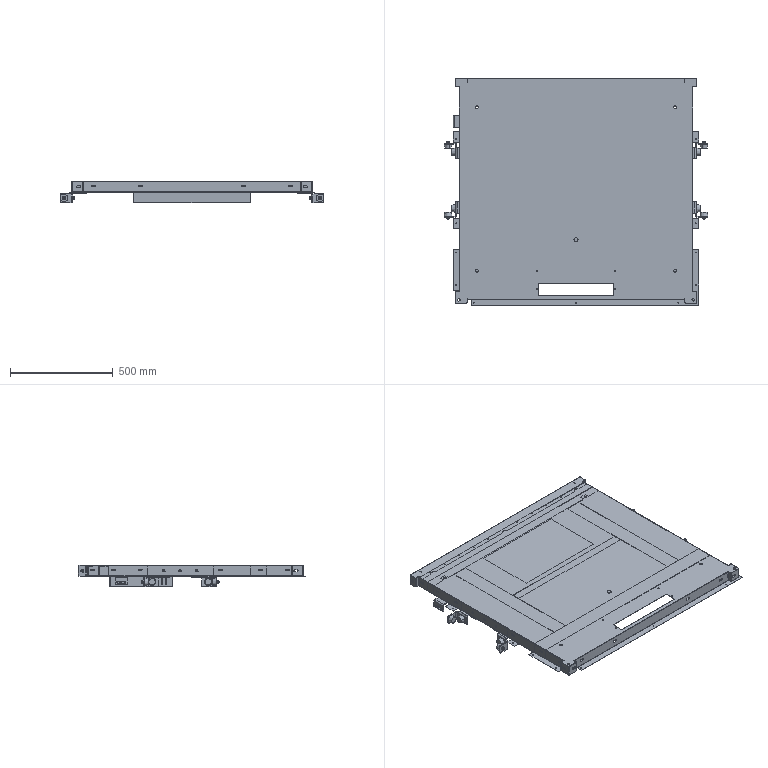Part | SolidWorks | features ReferencePattern 3, InContextFeatHolder 2, MirrorCompFeat 2 | 58 solids | 2088 faces | box 1282 x 1105 x 103.8 mm | volume 16071700 mm3 | plane 1277 | cylinder 635 | cone 168 | spline 8 | commonest cylinder face diameters 9 x76 6 x70 0.4 x62 10 x61 10.5 x60 3.4 x41